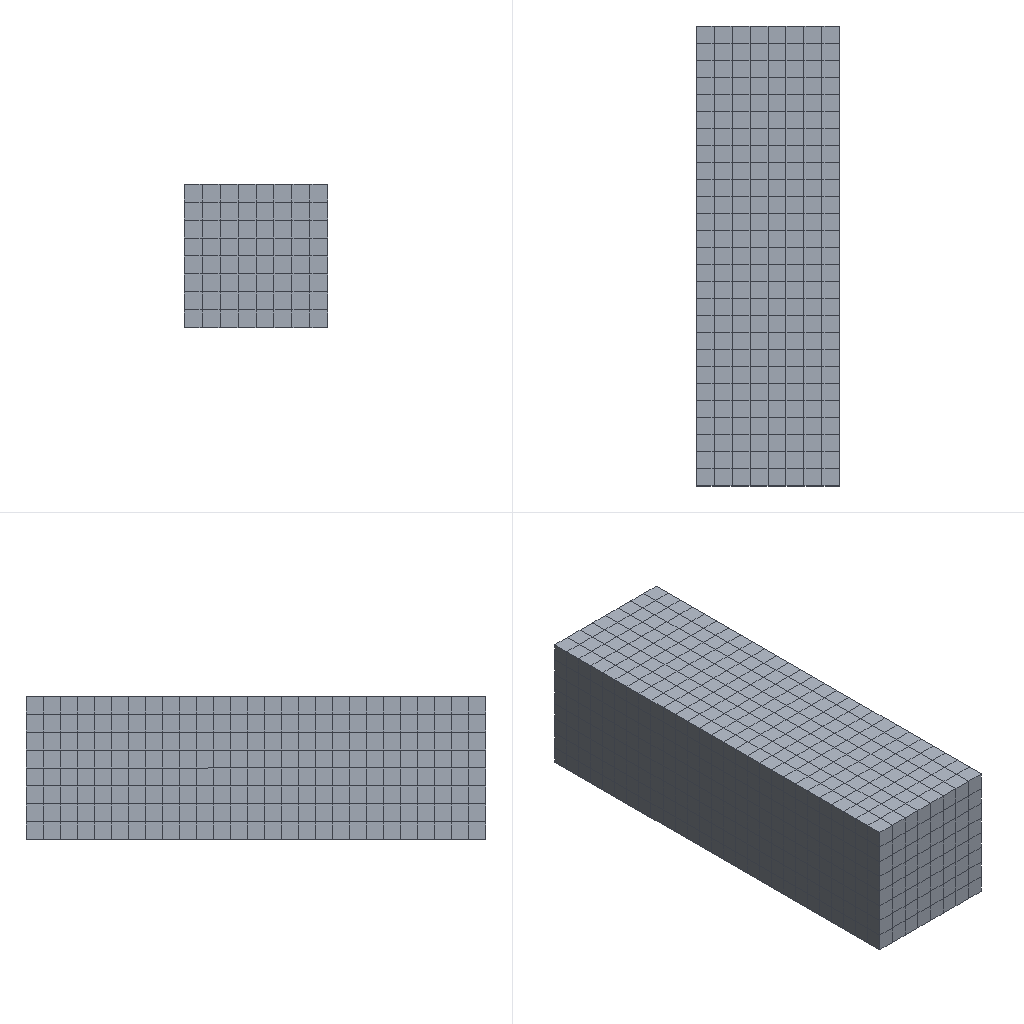Simulation study | abaqus
Set-up summary:
category,name,step,type,value,unit,region
solver,abaqus
solver,version,,,Abaqus/Explicit 2020
units,not stated in the deck,,not stated
analysis,deck,,transient,transient
load_step,Step-1,Step-1,transient
load_step,requested,,,1
mesh,nodes,,,3494
mesh,elements,,,2804
element_type,M3D4R,,membrane,1076
element_type,EC3D8R,,solid,1728
load,load commands in deck,,count,1
bc,support commands in deck,,count,8
material,AIR,,in results
material,MO,,in results
check,setup vs results,,match,"per instance, exact: element labels, types and connectivity; labels of the nodes the elements use; coordinates of those nodes at SINGLE_PRECISION in 1 of 2 instance(s)"
Abaqus input file, long lists of numbers shortened:
*Heading
** Job name: Job-1 Model name: Job-wurenji
** Generated by: Abaqus/CAE 2020
*Preprint, echo=NO, model=NO, history=NO, contact=NO
**
** PARTS
**
*Part, name=MO
*Node
      1,         -50.,  -1.987,          50.
      2,           0.,    8.013,          50.
** (1223 more lines like these left out)
*Element, type=M3D4R
   1,    1,   10,  202,   73
   2,   10,   11,  203,  202
** (1074 more lines like these left out)
*Node
   1226,           0.,           0.,          50.
*Nset, nset=MO-RefPt_, internal
1226,
*Nset, nset=_PICKEDSET4, internal, generate
    1,  1225,     1
*Elset, elset=_PICKEDSET4, internal
    1,    2,    3,    4,    5,    6,    7,    8,    9,   10,   11,   12,   18,   19,   20,   21
   22,   23,   24,   25,   26,   27,   28,   29,   35,   36,   37,   38,   39,   40,   41,   42
** (66 more lines like these left out)
** Section: Section-2-_PICKEDSET4
*Membrane Section, elset=_PICKEDSET4, material=MO
0.13,
*End Part
**
*Part, name=oulaair
*Node
      1,           0.,        -250.,         800.
      2,           0.,      -218.75,         800.
** (2266 more lines like these left out)
*Element, type=EC3D8R
   1,  253,  254,  263,  262,    1,    2,   11,   10
   2,  254,  255,  264,  263,    2,    3,   12,   11
** (1726 more lines like these left out)
*Nset, nset=Set-1, generate
    1,  2268,     1
*Elset, elset=Set-1, generate
    1,  1728,     1
** Section: Section-1-_PICKEDSET6
*Eulerian Section, elset=Set-1
AIR, AIR-1
*Surface, type=EULERIAN MATERIAL, name=AIR-1
AIR-1
*End Part
**
**
** ASSEMBLY
**
*Assembly, name=Assembly
**
*Instance, name=MO-1, part=MO
        125.,   -28.013,  -177.941
*End Instance
**
*Instance, name=oulaair-1, part=oulaair
          0.,           0.,           0.
          0.,           0.,           0., 1.,           0.,           0., 90.
*End Instance
**
*Node
      1, 1.79617961e-14,         950.,         500.
*Nset, nset=SET-RP1
 1,
*Nset, nset=Set-10, instance=MO-1
 1226,
*Elset, elset=Set-11, instance=MO-1
    1,    2,    3,    4,    5,    6,    7,    8,    9,   10,   11,   12,   18,   19,   20,   21
   22,   23,   24,   25,   26,   27,   28,   29,   35,   36,   37,   38,   39,   40,   41,   42
** (66 more lines like these left out)
*Nset, nset=Set-12, instance=MO-1, generate
    1,  1225,     1
*Nset, nset=Set-13, instance=oulaair-1
    1,    2,    3,    4,    5,    6,    7,    8,    9,  253,  254,  255,  256,  257,  258,  259
  260,  261,  505,  506,  507,  508,  509,  510,  511,  512,  513,  757,  758,  759,  760,  761
** (4 more lines like these left out)
*Elset, elset=Set-13, instance=oulaair-1
    1,    2,    3,    4,    5,    6,    7,    8,  217,  218,  219,  220,  221,  222,  223,  224
  433,  434,  435,  436,  437,  438,  439,  440,  649,  650,  651,  652,  653,  654,  655,  656
** (2 more lines like these left out)
*Nset, nset=Set-14, instance=oulaair-1
    1,    9,   10,   18,   19,   27,   28,   36,   37,   45,   46,   54,   55,   63,   64,   72
   73,   81,   82,   90,   91,   99,  100,  108,  109,  117,  118,  126,  127,  135,  136,  144
** (30 more lines like these left out)
*Elset, elset=Set-14, instance=oulaair-1
    1,    8,    9,   16,   17,   24,   25,   32,   33,   40,   41,   48,   49,   56,   57,   64
   65,   72,   73,   80,   81,   88,   89,   96,   97,  104,  105,  112,  113,  120,  121,  128
** (25 more lines like these left out)
*Nset, nset=Set-15, instance=oulaair-1
    1,    2,    3,    4,    5,    6,    7,    8,    9,   10,   11,   12,   13,   14,   15,   16
   17,   18,   19,   20,   21,   22,   23,   24,   25,   26,   27,   28,   29,   30,   31,   32
** (30 more lines like these left out)
*Elset, elset=Set-15, instance=oulaair-1
    1,    2,    3,    4,    5,    6,    7,    8,    9,   10,   11,   12,   13,   14,   15,   16
   17,   18,   19,   20,   21,   22,   23,   24,   25,   26,   27,   28,   29,   30,   31,   32
** (25 more lines like these left out)
*Nset, nset=Set-16, instance=MO-1
 1226,
*Elset, elset=b_Set-9, instance=MO-1
    1,    2,    3,    4,    5,    6,    7,    8,    9,   10,   11,   12,   18,   19,   20,   21
   22,   23,   24,   25,   26,   27,   28,   29,   35,   36,   37,   38,   39,   40,   41,   42
** (66 more lines like these left out)
*Nset, nset=t_Set-14, instance=MO-1
 4, 6, 8, 9
*Nset, nset=_PICKEDSET24, internal
 1,
*Nset, nset=_PICKEDSET31, internal
 1,
*Nset, nset=_PickedSet25, internal, instance=MO-1
 1226,
*Nset, nset=_PickedSet29, internal, instance=oulaair-1, generate
    1,  2268,     1
*Elset, elset=_PickedSet29, internal, instance=oulaair-1, generate
    1,  1728,     1
*Nset, nset=_PickedSet34, internal, instance=MO-1
 1226,
** Constraint: Constraint-2
*Rigid Body, ref node=_PickedSet34, tie nset=t_Set-14
*End Assembly
**
** MATERIALS
**
*Material, name=AIR
*Density
 1.204e-09,
*Eos, type=USUP
340000.,0.,0.
*Viscosity
 1.82e-10,
*Material, name=MO
*Density
 6.8886e-08,
*Elastic
100., 0.4
**
** INTERACTION PROPERTIES
**
*Surface Interaction, name=INTPROP-1
*Friction
 0.1,
*Surface Behavior, pressure-overclosure=HARD
**
** BOUNDARY CONDITIONS
**
** Name: BC-4 Type: 位移/转角
*Boundary
Set-16, 1, 1
Set-16, 3, 3
Set-16, 4, 4
Set-16, 5, 5
Set-16, 6, 6
**
** PREDEFINED FIELDS
**
** Name: Predefined Field-2   Type: Velocity
*Initial Conditions, type=VELOCITY
Set-12, 1, 0.
Set-12, 2, -570.
Set-12, 3, 0.
** Name: Predefined Field-3   Type: Material assignment
*Initial Conditions, type=VOLUME FRACTION
_PickedSet29, oulaair-1.AIR-1, 1.
**
** INTERACTIONS
**
** Interaction: general_contact
*Contact, op=NEW
*Contact Inclusions, ALL EXTERIOR
*Contact Property Assignment
 ,  , INTPROP-1
** ----------------------------------------------------------------
**
** STEP: Step-1
**
*Step, name=Step-1, nlgeom=YES
*Dynamic, Explicit
, 1.
*Bulk Viscosity
0.06, 1.2
** Mass Scaling: Semi-Automatic
**               Whole Model
*Fixed Mass Scaling, factor=50.
**
** BOUNDARY CONDITIONS
**
** Name: BC-1 Type: 位移/转角
*Boundary
Set-13, 2, 2
** Name: BC-2 Type: 位移/转角
*Boundary
Set-14, 3, 3
** Name: BC-3 Type: 位移/转角
*Boundary
Set-15, 1, 1
**
** OUTPUT REQUESTS
**
*Restart, write, number interval=1, time marks=NO
**
** FIELD OUTPUT: F-Output-1
**
*Output, field
*Node Output
A, U, V
**
** FIELD OUTPUT: F-Output-2
**
*Output, field, number interval=100
*Node Output
A, RF, RM, RT, U, V
*Element Output, directions=YES
DENSITYVAVG, E, EVF, EVOL, LE, MISES, MISESMAX, PE, PEEQ, PEEQMAX, PEEQT, PEMAG, PEVAVG, S, SSAVG, SVAVG
*Contact Output
CDISP, CSTRESS
*Output, history, frequency=0
*End Step
Results summary:
result,step,Step-1,completed,increments=21418 time=1.0/1.0
result,analysis,,,transient
result,last_loadstep,,,1
result,primary field,,,U
result,reaction total,,FX,-0.6291,model units
result,reaction total,,FY,-134.777,model units
result,reaction total,,FZ,-1.572,model units